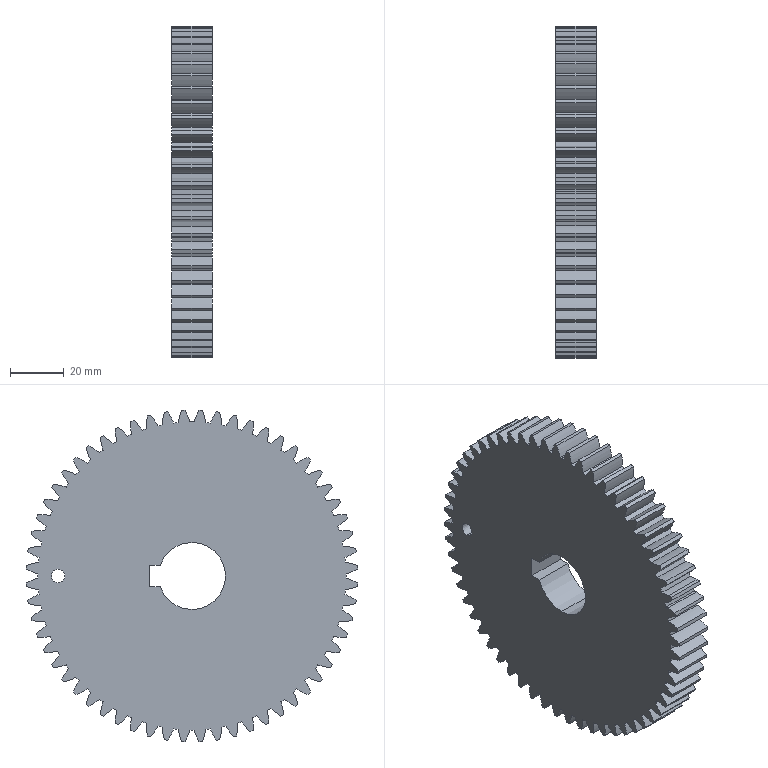Part | SolidWorks | features HoleWzd 1, MBimport 1 | 1 solid | 255 faces | box 15 x 123.892 x 123.892 mm | volume 159845 mm3 | cylinder 250 | plane 5 | commonest cylinder face diameters 48 x124 114.998 x61 124 x60 25 x3 5 x2